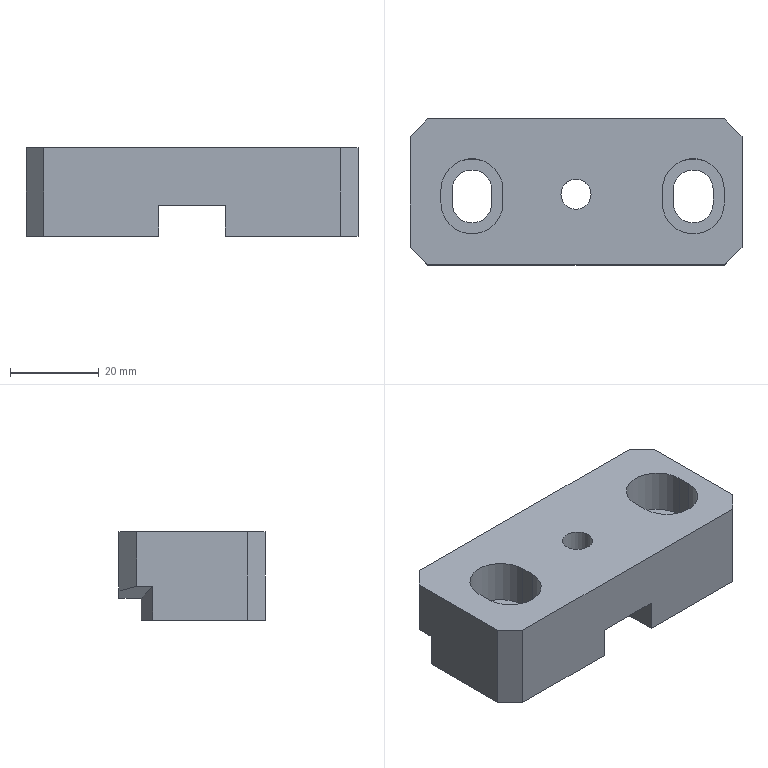Part | NX | features 20 2 | 1 solid | 41 faces | box 75 x 33 x 20 mm | volume 37493 mm3 | plane 32 | cylinder 9 | commonest cylinder face diameters 9 x4 14 x4 6.8 x1
STEP:
#1=CARTESIAN_POINT('',(1901.502,-433.5,16.5));
#2=VERTEX_POINT('',#1);
#3=CARTESIAN_POINT('',(1887.502,-433.5,16.5));
#4=VERTEX_POINT('',#3);
#5=CARTESIAN_POINT('',(1894.502,-433.5,16.5));
#6=DIRECTION('',(0.,0.,1.));
#7=DIRECTION('',(1.,0.,0.));
#8=AXIS2_PLACEMENT_3D('',#5,#6,#7);
#9=CIRCLE('',#8,7.);
#10=EDGE_CURVE('',#2,#4,#9,.T.);
#11=ORIENTED_EDGE('',*,*,#10,.F.);
#12=CARTESIAN_POINT('',(1901.502,-436.5,16.5));
#13=VERTEX_POINT('',#12);
#14=CARTESIAN_POINT('',(1901.502,-450.5,16.5));
#15=DIRECTION('',(0.,1.,0.));
#16=VECTOR('',#15,1000.);
#17=LINE('',#14,#16);
#18=EDGE_CURVE('',#13,#2,#17,.T.);
#19=ORIENTED_EDGE('',*,*,#18,.F.);
#20=CARTESIAN_POINT('',(1887.502,-436.5,16.5));
#21=VERTEX_POINT('',#20);
#22=CARTESIAN_POINT('',(1894.502,-436.5,16.5));
#23=DIRECTION('',(0.,0.,1.));
#24=DIRECTION('',(1.,0.,0.));
#25=AXIS2_PLACEMENT_3D('',#22,#23,#24);
#26=CIRCLE('',#25,7.);
#27=EDGE_CURVE('',#21,#13,#26,.T.);
#28=ORIENTED_EDGE('',*,*,#27,.F.);
#29=CARTESIAN_POINT('',(1887.502,-450.5,16.5));
#30=DIRECTION('',(0.,-1.,0.));
#31=VECTOR('',#30,1000.);
#32=LINE('',#29,#31);
#33=EDGE_CURVE('',#4,#21,#32,.T.);
#34=ORIENTED_EDGE('',*,*,#33,.F.);
#35=EDGE_LOOP('',(#11,#19,#28,#34));
#36=FACE_BOUND('',#35,.T.);
#37=CARTESIAN_POINT('',(1851.502,-436.5,16.5));
#38=VERTEX_POINT('',#37);
#39=CARTESIAN_POINT('',(1851.502,-433.5,16.5));
#40=VERTEX_POINT('',#39);
#41=CARTESIAN_POINT('',(1851.502,-450.5,16.5));
#42=DIRECTION('',(0.,1.,0.));
#43=VECTOR('',#42,1000.);
#44=LINE('',#41,#43);
#45=EDGE_CURVE('',#38,#40,#44,.T.);
#46=ORIENTED_EDGE('',*,*,#45,.F.);
#47=CARTESIAN_POINT('',(1837.502,-436.5,16.5));
#48=VERTEX_POINT('',#47);
#49=CARTESIAN_POINT('',(1844.502,-436.5,16.5));
#50=DIRECTION('',(0.,0.,1.));
#51=DIRECTION('',(1.,0.,0.));
#52=AXIS2_PLACEMENT_3D('',#49,#50,#51);
#53=CIRCLE('',#52,7.);
#54=EDGE_CURVE('',#48,#38,#53,.T.);
#55=ORIENTED_EDGE('',*,*,#54,.F.);
#56=CARTESIAN_POINT('',(1837.502,-433.5,16.5));
#57=VERTEX_POINT('',#56);
#58=CARTESIAN_POINT('',(1837.502,-450.5,16.5));
#59=DIRECTION('',(0.,-1.,0.));
#60=VECTOR('',#59,1000.);
#61=LINE('',#58,#60);
#62=EDGE_CURVE('',#57,#48,#61,.T.);
#63=ORIENTED_EDGE('',*,*,#62,.F.);
#64=CARTESIAN_POINT('',(1844.502,-433.5,16.5));
#65=DIRECTION('',(0.,0.,1.));
#66=DIRECTION('',(1.,0.,0.));
#67=AXIS2_PLACEMENT_3D('',#64,#65,#66);
#68=CIRCLE('',#67,7.);
#69=EDGE_CURVE('',#40,#57,#68,.T.);
#70=ORIENTED_EDGE('',*,*,#69,.F.);
#71=EDGE_LOOP('',(#46,#55,#63,#70));
#72=FACE_BOUND('',#71,.T.);
#73=CARTESIAN_POINT('',(1901.502,-417.5,16.5));
#74=VERTEX_POINT('',#73);
#75=CARTESIAN_POINT('',(1834.502,-417.5,16.5));
#76=VERTEX_POINT('',#75);
#77=CARTESIAN_POINT('',(1968.502,-417.5,16.5));
#78=DIRECTION('',(-1.,0.,0.));
#79=VECTOR('',#78,1000.);
#80=LINE('',#77,#79);
#81=EDGE_CURVE('',#74,#76,#80,.T.);
#82=ORIENTED_EDGE('',*,*,#81,.T.);
#83=CARTESIAN_POINT('',(1830.502,-421.5,16.5));
#84=VERTEX_POINT('',#83);
#85=CARTESIAN_POINT('',(1830.502,-421.5,16.5));
#86=DIRECTION('',(-0.7071,-0.7071,0.));
#87=VECTOR('',#86,1000.);
#88=LINE('',#85,#87);
#89=EDGE_CURVE('',#76,#84,#88,.T.);
#90=ORIENTED_EDGE('',*,*,#89,.T.);
#91=CARTESIAN_POINT('',(1830.502,-446.5,16.5));
#92=VERTEX_POINT('',#91);
#93=CARTESIAN_POINT('',(1830.502,-417.5,16.5));
#94=DIRECTION('',(0.,-1.,0.));
#95=VECTOR('',#94,1000.);
#96=LINE('',#93,#95);
#97=EDGE_CURVE('',#84,#92,#96,.T.);
#98=ORIENTED_EDGE('',*,*,#97,.T.);
#99=CARTESIAN_POINT('',(1834.502,-450.5,16.5));
#100=VERTEX_POINT('',#99);
#101=CARTESIAN_POINT('',(1834.502,-450.5,16.5));
#102=DIRECTION('',(0.7071,-0.7071,0.));
#103=VECTOR('',#102,1000.);
#104=LINE('',#101,#103);
#105=EDGE_CURVE('',#92,#100,#104,.T.);
#106=ORIENTED_EDGE('',*,*,#105,.T.);
#107=CARTESIAN_POINT('',(1901.502,-450.5,16.5));
#108=VERTEX_POINT('',#107);
#109=CARTESIAN_POINT('',(1888.502,-450.5,16.5));
#110=DIRECTION('',(1.,0.,0.));
#111=VECTOR('',#110,1000.);
#112=LINE('',#109,#111);
#113=EDGE_CURVE('',#100,#108,#112,.T.);
#114=ORIENTED_EDGE('',*,*,#113,.T.);
#115=CARTESIAN_POINT('',(1905.502,-446.5,16.5));
#116=VERTEX_POINT('',#115);
#117=CARTESIAN_POINT('',(1905.502,-446.5,16.5));
#118=DIRECTION('',(0.7071,0.7071,0.));
#119=VECTOR('',#118,1000.);
#120=LINE('',#117,#119);
#121=EDGE_CURVE('',#108,#116,#120,.T.);
#122=ORIENTED_EDGE('',*,*,#121,.T.);
#123=CARTESIAN_POINT('',(1905.502,-421.5,16.5));
#124=VERTEX_POINT('',#123);
#125=CARTESIAN_POINT('',(1905.502,-450.5,16.5));
#126=DIRECTION('',(0.,1.,0.));
#127=VECTOR('',#126,1000.);
#128=LINE('',#125,#127);
#129=EDGE_CURVE('',#116,#124,#128,.T.);
#130=ORIENTED_EDGE('',*,*,#129,.T.);
#131=CARTESIAN_POINT('',(1901.502,-417.5,16.5));
#132=DIRECTION('',(-0.7071,0.7071,0.));
#133=VECTOR('',#132,1000.);
#134=LINE('',#131,#133);
#135=EDGE_CURVE('',#124,#74,#134,.T.);
#136=ORIENTED_EDGE('',*,*,#135,.T.);
#137=EDGE_LOOP('',(#82,#90,#98,#106,#114,#122,#130,#136));
#138=FACE_BOUND('',#137,.T.);
#139=CARTESIAN_POINT('',(1871.402,-434.5,16.5));
#140=VERTEX_POINT('',#139);
#141=CARTESIAN_POINT('',(1868.002,-434.5,16.5));
#142=DIRECTION('',(0.,0.,-1.));
#143=DIRECTION('',(1.,0.,0.));
#144=AXIS2_PLACEMENT_3D('',#141,#142,#143);
#145=CIRCLE('',#144,3.4);
#146=EDGE_CURVE('',#140,#140,#145,.T.);
#147=ORIENTED_EDGE('',*,*,#146,.T.);
#148=EDGE_LOOP('',(#147));
#149=FACE_BOUND('',#148,.T.);
#150=CARTESIAN_POINT('',(1968.502,-450.5,16.5));
#151=DIRECTION('',(0.,0.,1.));
#152=DIRECTION('',(-1.,0.,0.));
#153=AXIS2_PLACEMENT_3D('',#150,#151,#152);
#154=PLANE('',#153);
#155=ADVANCED_FACE('',(#36,#72,#138,#149),#154,.T.);
#156=CARTESIAN_POINT('',(1875.502,-417.5,3.5));
#157=VERTEX_POINT('',#156);
#158=CARTESIAN_POINT('',(1875.502,-450.5,3.5));
#159=VERTEX_POINT('',#158);
#160=CARTESIAN_POINT('',(1875.502,-436.5,3.5));
#161=DIRECTION('',(0.,-1.,0.));
#162=VECTOR('',#161,1000.);
#163=LINE('',#160,#162);
#164=EDGE_CURVE('',#157,#159,#163,.T.);
#165=ORIENTED_EDGE('',*,*,#164,.F.);
#166=CARTESIAN_POINT('',(1875.502,-417.5,1.5));
#167=VERTEX_POINT('',#166);
#168=CARTESIAN_POINT('',(1875.502,-417.5,11.5));
#169=DIRECTION('',(0.,0.,-1.));
#170=VECTOR('',#169,1000.);
#171=LINE('',#168,#170);
#172=EDGE_CURVE('',#157,#167,#171,.T.);
#173=ORIENTED_EDGE('',*,*,#172,.T.);
#174=CARTESIAN_POINT('',(1875.502,-422.5,1.5));
#175=VERTEX_POINT('',#174);
#176=CARTESIAN_POINT('',(1875.502,-396.891,1.5));
#177=DIRECTION('',(0.,1.,0.));
#178=VECTOR('',#177,1000.);
#179=LINE('',#176,#178);
#180=EDGE_CURVE('',#175,#167,#179,.T.);
#181=ORIENTED_EDGE('',*,*,#180,.F.);
#182=CARTESIAN_POINT('',(1875.502,-422.5,-3.5));
#183=VERTEX_POINT('',#182);
#184=CARTESIAN_POINT('',(1875.502,-422.5,3.5));
#185=DIRECTION('',(0.,0.,-1.));
#186=VECTOR('',#185,1000.);
#187=LINE('',#184,#186);
#188=EDGE_CURVE('',#175,#183,#187,.T.);
#189=ORIENTED_EDGE('',*,*,#188,.T.);
#190=CARTESIAN_POINT('',(1875.502,-450.5,-3.5));
#191=VERTEX_POINT('',#190);
#192=CARTESIAN_POINT('',(1875.502,-450.5,-3.5));
#193=DIRECTION('',(0.,-1.,0.));
#194=VECTOR('',#193,1000.);
#195=LINE('',#192,#194);
#196=EDGE_CURVE('',#183,#191,#195,.T.);
#197=ORIENTED_EDGE('',*,*,#196,.T.);
#198=CARTESIAN_POINT('',(1875.502,-450.5,11.5));
#199=DIRECTION('',(0.,0.,1.));
#200=VECTOR('',#199,1000.);
#201=LINE('',#198,#200);
#202=EDGE_CURVE('',#191,#159,#201,.T.);
#203=ORIENTED_EDGE('',*,*,#202,.T.);
#204=EDGE_LOOP('',(#165,#173,#181,#189,#197,#203));
#205=FACE_BOUND('',#204,.T.);
#206=CARTESIAN_POINT('',(1875.502,-436.5,0.));
#207=DIRECTION('',(-1.,0.,0.));
#208=DIRECTION('',(0.,0.,1.));
#209=AXIS2_PLACEMENT_3D('',#206,#207,#208);
#210=PLANE('',#209);
#211=ADVANCED_FACE('',(#205),#210,.T.);
#212=CARTESIAN_POINT('',(1860.502,-422.5,-3.5));
#213=VERTEX_POINT('',#212);
#214=CARTESIAN_POINT('',(1860.502,-450.5,-3.5));
#215=VERTEX_POINT('',#214);
#216=CARTESIAN_POINT('',(1860.502,-450.5,-3.5));
#217=DIRECTION('',(0.,-1.,0.));
#218=VECTOR('',#217,1000.);
#219=LINE('',#216,#218);
#220=EDGE_CURVE('',#213,#215,#219,.T.);
#221=ORIENTED_EDGE('',*,*,#220,.F.);
#222=CARTESIAN_POINT('',(1860.502,-422.5,1.5));
#223=VERTEX_POINT('',#222);
#224=CARTESIAN_POINT('',(1860.502,-422.5,3.5));
#225=DIRECTION('',(0.,0.,-1.));
#226=VECTOR('',#225,1000.);
#227=LINE('',#224,#226);
#228=EDGE_CURVE('',#223,#213,#227,.T.);
#229=ORIENTED_EDGE('',*,*,#228,.F.);
#230=CARTESIAN_POINT('',(1860.502,-417.5,1.5));
#231=VERTEX_POINT('',#230);
#232=CARTESIAN_POINT('',(1860.502,-396.891,1.5));
#233=DIRECTION('',(0.,1.,0.));
#234=VECTOR('',#233,1000.);
#235=LINE('',#232,#234);
#236=EDGE_CURVE('',#223,#231,#235,.T.);
#237=ORIENTED_EDGE('',*,*,#236,.T.);
#238=CARTESIAN_POINT('',(1860.502,-417.5,3.5));
#239=VERTEX_POINT('',#238);
#240=CARTESIAN_POINT('',(1860.502,-417.5,11.5));
#241=DIRECTION('',(0.,0.,-1.));
#242=VECTOR('',#241,1000.);
#243=LINE('',#240,#242);
#244=EDGE_CURVE('',#239,#231,#243,.T.);
#245=ORIENTED_EDGE('',*,*,#244,.F.);
#246=CARTESIAN_POINT('',(1860.502,-450.5,3.5));
#247=VERTEX_POINT('',#246);
#248=CARTESIAN_POINT('',(1860.502,-436.5,3.5));
#249=DIRECTION('',(0.,1.,0.));
#250=VECTOR('',#249,1000.);
#251=LINE('',#248,#250);
#252=EDGE_CURVE('',#247,#239,#251,.T.);
#253=ORIENTED_EDGE('',*,*,#252,.F.);
#254=CARTESIAN_POINT('',(1860.502,-450.5,11.5));
#255=DIRECTION('',(0.,0.,1.));
#256=VECTOR('',#255,1000.);
#257=LINE('',#254,#256);
#258=EDGE_CURVE('',#215,#247,#257,.T.);
#259=ORIENTED_EDGE('',*,*,#258,.F.);
#260=EDGE_LOOP('',(#221,#229,#237,#245,#253,#259));
#261=FACE_BOUND('',#260,.T.);
#262=CARTESIAN_POINT('',(1860.502,-436.5,-9.5));
#263=DIRECTION('',(-1.,0.,0.));
#264=DIRECTION('',(0.,0.,-1.));
#265=AXIS2_PLACEMENT_3D('',#262,#263,#264);
#266=PLANE('',#265);
#267=ADVANCED_FACE('',(#261),#266,.F.);
#268=CARTESIAN_POINT('',(1871.402,-434.5,3.5));
#269=VERTEX_POINT('',#268);
#270=CARTESIAN_POINT('',(1868.002,-434.5,3.5));
#271=DIRECTION('',(0.,0.,1.));
#272=DIRECTION('',(1.,0.,0.));
#273=AXIS2_PLACEMENT_3D('',#270,#271,#272);
#274=CIRCLE('',#273,3.4);
#275=EDGE_CURVE('',#269,#269,#274,.T.);
#276=ORIENTED_EDGE('',*,*,#275,.T.);
#277=EDGE_LOOP('',(#276));
#278=FACE_BOUND('',#277,.T.);
#279=CARTESIAN_POINT('',(1938.502,-450.5,3.5));
#280=DIRECTION('',(1.,0.,0.));
#281=VECTOR('',#280,1000.);
#282=LINE('',#279,#281);
#283=EDGE_CURVE('',#247,#159,#282,.T.);
#284=ORIENTED_EDGE('',*,*,#283,.F.);
#285=ORIENTED_EDGE('',*,*,#252,.T.);
#286=CARTESIAN_POINT('',(2018.502,-417.5,3.5));
#287=DIRECTION('',(-1.,0.,0.));
#288=VECTOR('',#287,1000.);
#289=LINE('',#286,#288);
#290=EDGE_CURVE('',#157,#239,#289,.T.);
#291=ORIENTED_EDGE('',*,*,#290,.F.);
#292=ORIENTED_EDGE('',*,*,#164,.T.);
#293=EDGE_LOOP('',(#284,#285,#291,#292));
#294=FACE_BOUND('',#293,.T.);
#295=CARTESIAN_POINT('',(1868.002,-436.5,3.5));
#296=DIRECTION('',(0.,0.,1.));
#297=DIRECTION('',(0.,-1.,0.));
#298=AXIS2_PLACEMENT_3D('',#295,#296,#297);
#299=PLANE('',#298);
#300=ADVANCED_FACE('',(#278,#294),#299,.F.);
#301=CARTESIAN_POINT('',(1890.002,-436.5,6.5));
#302=VERTEX_POINT('',#301);
#303=CARTESIAN_POINT('',(1890.002,-433.5,6.5));
#304=VERTEX_POINT('',#303);
#305=CARTESIAN_POINT('',(1890.002,-432.5,6.5));
#306=DIRECTION('',(0.,1.,0.));
#307=VECTOR('',#306,1000.);
#308=LINE('',#305,#307);
#309=EDGE_CURVE('',#302,#304,#308,.T.);
#310=ORIENTED_EDGE('',*,*,#309,.T.);
#311=CARTESIAN_POINT('',(1899.002,-433.5,6.5));
#312=VERTEX_POINT('',#311);
#313=CARTESIAN_POINT('',(1894.502,-433.5,6.5));
#314=DIRECTION('',(0.,0.,-1.));
#315=DIRECTION('',(-1.,0.,0.));
#316=AXIS2_PLACEMENT_3D('',#313,#314,#315);
#317=CIRCLE('',#316,4.5);
#318=EDGE_CURVE('',#304,#312,#317,.T.);
#319=ORIENTED_EDGE('',*,*,#318,.T.);
#320=CARTESIAN_POINT('',(1899.002,-436.5,6.5));
#321=VERTEX_POINT('',#320);
#322=CARTESIAN_POINT('',(1899.002,-439.5,6.5));
#323=DIRECTION('',(0.,-1.,0.));
#324=VECTOR('',#323,1000.);
#325=LINE('',#322,#324);
#326=EDGE_CURVE('',#312,#321,#325,.T.);
#327=ORIENTED_EDGE('',*,*,#326,.T.);
#328=CARTESIAN_POINT('',(1894.502,-436.5,6.5));
#329=DIRECTION('',(0.,0.,-1.));
#330=DIRECTION('',(-1.,0.,0.));
#331=AXIS2_PLACEMENT_3D('',#328,#329,#330);
#332=CIRCLE('',#331,4.5);
#333=EDGE_CURVE('',#321,#302,#332,.T.);
#334=ORIENTED_EDGE('',*,*,#333,.T.);
#335=EDGE_LOOP('',(#310,#319,#327,#334));
#336=FACE_BOUND('',#335,.T.);
#337=CARTESIAN_POINT('',(1901.502,-433.5,6.5));
#338=VERTEX_POINT('',#337);
#339=CARTESIAN_POINT('',(1887.502,-433.5,6.5));
#340=VERTEX_POINT('',#339);
#341=CARTESIAN_POINT('',(1894.502,-433.5,6.5));
#342=DIRECTION('',(0.,0.,1.));
#343=DIRECTION('',(-1.,0.,0.));
#344=AXIS2_PLACEMENT_3D('',#341,#342,#343);
#345=CIRCLE('',#344,7.);
#346=EDGE_CURVE('',#338,#340,#345,.T.);
#347=ORIENTED_EDGE('',*,*,#346,.T.);
#348=CARTESIAN_POINT('',(1887.502,-436.5,6.5));
#349=VERTEX_POINT('',#348);
#350=CARTESIAN_POINT('',(1887.502,-439.5,6.5));
#351=DIRECTION('',(0.,-1.,0.));
#352=VECTOR('',#351,1000.);
#353=LINE('',#350,#352);
#354=EDGE_CURVE('',#340,#349,#353,.T.);
#355=ORIENTED_EDGE('',*,*,#354,.T.);
#356=CARTESIAN_POINT('',(1901.502,-436.5,6.5));
#357=VERTEX_POINT('',#356);
#358=CARTESIAN_POINT('',(1894.502,-436.5,6.5));
#359=DIRECTION('',(0.,0.,1.));
#360=DIRECTION('',(-1.,0.,0.));
#361=AXIS2_PLACEMENT_3D('',#358,#359,#360);
#362=CIRCLE('',#361,7.);
#363=EDGE_CURVE('',#349,#357,#362,.T.);
#364=ORIENTED_EDGE('',*,*,#363,.T.);
#365=CARTESIAN_POINT('',(1901.502,-432.5,6.5));
#366=DIRECTION('',(0.,1.,0.));
#367=VECTOR('',#366,1000.);
#368=LINE('',#365,#367);
#369=EDGE_CURVE('',#357,#338,#368,.T.);
#370=ORIENTED_EDGE('',*,*,#369,.T.);
#371=EDGE_LOOP('',(#347,#355,#364,#370));
#372=FACE_BOUND('',#371,.T.);
#373=CARTESIAN_POINT('',(1894.502,-432.5,6.5));
#374=DIRECTION('',(0.,0.,-1.));
#375=DIRECTION('',(1.,0.,0.));
#376=AXIS2_PLACEMENT_3D('',#373,#374,#375);
#377=PLANE('',#376);
#378=ADVANCED_FACE('',(#336,#372),#377,.F.);
#379=CARTESIAN_POINT('',(1895.502,-417.5,1.5));
#380=VERTEX_POINT('',#379);
#381=CARTESIAN_POINT('',(1895.502,-422.5,1.5));
#382=VERTEX_POINT('',#381);
#383=CARTESIAN_POINT('',(1895.502,-425.18,1.5));
#384=DIRECTION('',(0.,-1.,0.));
#385=VECTOR('',#384,1000.);
#386=LINE('',#383,#385);
#387=EDGE_CURVE('',#380,#382,#386,.T.);
#388=ORIENTED_EDGE('',*,*,#387,.F.);
#389=CARTESIAN_POINT('',(1901.502,-417.5,3.108));
#390=VERTEX_POINT('',#389);
#391=CARTESIAN_POINT('',(1895.502,-417.5,1.5));
#392=DIRECTION('',(-0.9659,0.,-0.2588));
#393=VECTOR('',#392,1000.);
#394=LINE('',#391,#393);
#395=EDGE_CURVE('',#390,#380,#394,.T.);
#396=ORIENTED_EDGE('',*,*,#395,.F.);
#397=CARTESIAN_POINT('',(1905.502,-421.5,4.179));
#398=VERTEX_POINT('',#397);
#399=CARTESIAN_POINT('',(1888.451,-404.449,-0.3894));
#400=DIRECTION('',(0.6947,-0.6947,0.1862));
#401=VECTOR('',#400,1000.);
#402=LINE('',#399,#401);
#403=EDGE_CURVE('',#390,#398,#402,.T.);
#404=ORIENTED_EDGE('',*,*,#403,.T.);
#405=CARTESIAN_POINT('',(1905.502,-425.18,4.179));
#406=VERTEX_POINT('',#405);
#407=CARTESIAN_POINT('',(1905.502,-417.5,4.179));
#408=DIRECTION('',(0.,1.,0.));
#409=VECTOR('',#408,1000.);
#410=LINE('',#407,#409);
#411=EDGE_CURVE('',#406,#398,#410,.T.);
#412=ORIENTED_EDGE('',*,*,#411,.F.);
#413=CARTESIAN_POINT('',(1904.875,-425.012,4.011));
#414=DIRECTION('',(0.9351,-0.2506,0.2506));
#415=VECTOR('',#414,1000.);
#416=LINE('',#413,#415);
#417=EDGE_CURVE('',#382,#406,#416,.T.);
#418=ORIENTED_EDGE('',*,*,#417,.F.);
#419=EDGE_LOOP('',(#388,#396,#404,#412,#418));
#420=FACE_BOUND('',#419,.T.);
#421=CARTESIAN_POINT('',(1895.502,-396.891,1.5));
#422=DIRECTION('',(0.2588,0.,-0.9659));
#423=DIRECTION('',(0.9659,0.,0.2588));
#424=AXIS2_PLACEMENT_3D('',#421,#422,#423);
#425=PLANE('',#424);
#426=ADVANCED_FACE('',(#420),#425,.T.);
#427=CARTESIAN_POINT('',(1849.002,-433.5,6.5));
#428=VERTEX_POINT('',#427);
#429=CARTESIAN_POINT('',(1849.002,-436.5,6.5));
#430=VERTEX_POINT('',#429);
#431=CARTESIAN_POINT('',(1849.002,-432.5,6.5));
#432=DIRECTION('',(0.,-1.,0.));
#433=VECTOR('',#432,1000.);
#434=LINE('',#431,#433);
#435=EDGE_CURVE('',#428,#430,#434,.T.);
#436=ORIENTED_EDGE('',*,*,#435,.T.);
#437=CARTESIAN_POINT('',(1840.002,-436.5,6.5));
#438=VERTEX_POINT('',#437);
#439=CARTESIAN_POINT('',(1844.502,-436.5,6.5));
#440=DIRECTION('',(0.,0.,-1.));
#441=DIRECTION('',(-1.,0.,0.));
#442=AXIS2_PLACEMENT_3D('',#439,#440,#441);
#443=CIRCLE('',#442,4.5);
#444=EDGE_CURVE('',#430,#438,#443,.T.);
#445=ORIENTED_EDGE('',*,*,#444,.T.);
#446=CARTESIAN_POINT('',(1840.002,-433.5,6.5));
#447=VERTEX_POINT('',#446);
#448=CARTESIAN_POINT('',(1840.002,-439.5,6.5));
#449=DIRECTION('',(0.,1.,0.));
#450=VECTOR('',#449,1000.);
#451=LINE('',#448,#450);
#452=EDGE_CURVE('',#438,#447,#451,.T.);
#453=ORIENTED_EDGE('',*,*,#452,.T.);
#454=CARTESIAN_POINT('',(1844.502,-433.5,6.5));
#455=DIRECTION('',(0.,0.,-1.));
#456=DIRECTION('',(-1.,0.,0.));
#457=AXIS2_PLACEMENT_3D('',#454,#455,#456);
#458=CIRCLE('',#457,4.5);
#459=EDGE_CURVE('',#447,#428,#458,.T.);
#460=ORIENTED_EDGE('',*,*,#459,.T.);
#461=EDGE_LOOP('',(#436,#445,#453,#460));
#462=FACE_BOUND('',#461,.T.);
#463=CARTESIAN_POINT('',(1851.502,-433.5,6.5));
#464=VERTEX_POINT('',#463);
#465=CARTESIAN_POINT('',(1837.502,-433.5,6.5));
#466=VERTEX_POINT('',#465);
#467=CARTESIAN_POINT('',(1844.502,-433.5,6.5));
#468=DIRECTION('',(0.,0.,1.));
#469=DIRECTION('',(-1.,0.,0.));
#470=AXIS2_PLACEMENT_3D('',#467,#468,#469);
#471=CIRCLE('',#470,7.);
#472=EDGE_CURVE('',#464,#466,#471,.T.);
#473=ORIENTED_EDGE('',*,*,#472,.T.);
#474=CARTESIAN_POINT('',(1837.502,-436.5,6.5));
#475=VERTEX_POINT('',#474);
#476=CARTESIAN_POINT('',(1837.502,-432.5,6.5));
#477=DIRECTION('',(0.,-1.,0.));
#478=VECTOR('',#477,1000.);
#479=LINE('',#476,#478);
#480=EDGE_CURVE('',#466,#475,#479,.T.);
#481=ORIENTED_EDGE('',*,*,#480,.T.);
#482=CARTESIAN_POINT('',(1851.502,-436.5,6.5));
#483=VERTEX_POINT('',#482);
#484=CARTESIAN_POINT('',(1844.502,-436.5,6.5));
#485=DIRECTION('',(0.,0.,1.));
#486=DIRECTION('',(-1.,0.,0.));
#487=AXIS2_PLACEMENT_3D('',#484,#485,#486);
#488=CIRCLE('',#487,7.);
#489=EDGE_CURVE('',#475,#483,#488,.T.);
#490=ORIENTED_EDGE('',*,*,#489,.T.);
#491=CARTESIAN_POINT('',(1851.502,-439.5,6.5));
#492=DIRECTION('',(0.,1.,0.));
#493=VECTOR('',#492,1000.);
#494=LINE('',#491,#493);
#495=EDGE_CURVE('',#483,#464,#494,.T.);
#496=ORIENTED_EDGE('',*,*,#495,.T.);
#497=EDGE_LOOP('',(#473,#481,#490,#496));
#498=FACE_BOUND('',#497,.T.);
#499=CARTESIAN_POINT('',(1844.502,-432.5,6.5));
#500=DIRECTION('',(0.,0.,-1.));
#501=DIRECTION('',(-1.,0.,0.));
#502=AXIS2_PLACEMENT_3D('',#499,#500,#501);
#503=PLANE('',#502);
#504=ADVANCED_FACE('',(#462,#498),#503,.F.);
#505=ORIENTED_EDGE('',*,*,#33,.T.);
#506=CARTESIAN_POINT('',(1887.502,-436.5,42.5));
#507=DIRECTION('',(0.,0.,1.));
#508=VECTOR('',#507,1000.);
#509=LINE('',#506,#508);
#510=EDGE_CURVE('',#349,#21,#509,.T.);
#511=ORIENTED_EDGE('',*,*,#510,.F.);
#512=ORIENTED_EDGE('',*,*,#354,.F.);
#513=CARTESIAN_POINT('',(1887.502,-433.5,42.5));
#514=DIRECTION('',(0.,0.,1.));
#515=VECTOR('',#514,1000.);
#516=LINE('',#513,#515);
#517=EDGE_CURVE('',#340,#4,#516,.T.);
#518=ORIENTED_EDGE('',*,*,#517,.T.);
#519=EDGE_LOOP('',(#505,#511,#512,#518));
#520=FACE_BOUND('',#519,.T.);
#521=CARTESIAN_POINT('',(1887.502,-439.5,42.5));
#522=DIRECTION('',(-1.,0.,0.));
#523=DIRECTION('',(0.,0.,-1.));
#524=AXIS2_PLACEMENT_3D('',#521,#522,#523);
#525=PLANE('',#524);
#526=ADVANCED_FACE('',(#520),#525,.F.);
#527=ORIENTED_EDGE('',*,*,#27,.T.);
#528=CARTESIAN_POINT('',(1901.502,-436.5,42.5));
#529=DIRECTION('',(0.,0.,1.));
#530=VECTOR('',#529,1000.);
#531=LINE('',#528,#530);
#532=EDGE_CURVE('',#357,#13,#531,.T.);
#533=ORIENTED_EDGE('',*,*,#532,.F.);
#534=ORIENTED_EDGE('',*,*,#363,.F.);
#535=ORIENTED_EDGE('',*,*,#510,.T.);
#536=EDGE_LOOP('',(#527,#533,#534,#535));
#537=FACE_BOUND('',#536,.T.);
#538=CARTESIAN_POINT('',(1894.502,-436.5,42.5));
#539=DIRECTION('',(0.,0.,-1.));
#540=DIRECTION('',(1.,0.,0.));
#541=AXIS2_PLACEMENT_3D('',#538,#539,#540);
#542=CYLINDRICAL_SURFACE('',#541,7.);
#543=ADVANCED_FACE('',(#537),#542,.F.);
#544=ORIENTED_EDGE('',*,*,#18,.T.);
#545=CARTESIAN_POINT('',(1901.502,-433.5,42.5));
#546=DIRECTION('',(0.,0.,1.));
#547=VECTOR('',#546,1000.);
#548=LINE('',#545,#547);
#549=EDGE_CURVE('',#338,#2,#548,.T.);
#550=ORIENTED_EDGE('',*,*,#549,.F.);
#551=ORIENTED_EDGE('',*,*,#369,.F.);
#552=ORIENTED_EDGE('',*,*,#532,.T.);
#553=EDGE_LOOP('',(#544,#550,#551,#552));
#554=FACE_BOUND('',#553,.T.);
#555=CARTESIAN_POINT('',(1901.502,-432.5,42.5));
#556=DIRECTION('',(1.,0.,0.));
#557=DIRECTION('',(0.,0.,1.));
#558=AXIS2_PLACEMENT_3D('',#555,#556,#557);
#559=PLANE('',#558);
#560=ADVANCED_FACE('',(#554),#559,.F.);
#561=ORIENTED_EDGE('',*,*,#10,.T.);
#562=ORIENTED_EDGE('',*,*,#517,.F.);
#563=ORIENTED_EDGE('',*,*,#346,.F.);
#564=ORIENTED_EDGE('',*,*,#549,.T.);
#565=EDGE_LOOP('',(#561,#562,#563,#564));
#566=FACE_BOUND('',#565,.T.);
#567=CARTESIAN_POINT('',(1894.502,-433.5,42.5));
#568=DIRECTION('',(0.,0.,-1.));
#569=DIRECTION('',(1.,0.,0.));
#570=AXIS2_PLACEMENT_3D('',#567,#568,#569);
#571=CYLINDRICAL_SURFACE('',#570,7.);
#572=ADVANCED_FACE('',(#566),#571,.F.);
#573=ORIENTED_EDGE('',*,*,#135,.F.);
#574=CARTESIAN_POINT('',(1905.502,-421.5,11.5));
#575=DIRECTION('',(0.,0.,1.));
#576=VECTOR('',#575,1000.);
#577=LINE('',#574,#576);
#578=EDGE_CURVE('',#398,#124,#577,.T.);
#579=ORIENTED_EDGE('',*,*,#578,.F.);
#580=ORIENTED_EDGE('',*,*,#403,.F.);
#581=CARTESIAN_POINT('',(1901.502,-417.5,11.5));
#582=DIRECTION('',(0.,0.,-1.));
#583=VECTOR('',#582,1000.);
#584=LINE('',#581,#583);
#585=EDGE_CURVE('',#74,#390,#584,.T.);
#586=ORIENTED_EDGE('',*,*,#585,.F.);
#587=EDGE_LOOP('',(#573,#579,#580,#586));
#588=FACE_BOUND('',#587,.T.);
#589=CARTESIAN_POINT('',(1901.502,-417.5,11.5));
#590=DIRECTION('',(-0.7071,-0.7071,0.));
#591=DIRECTION('',(0.,0.,-1.));
#592=AXIS2_PLACEMENT_3D('',#589,#590,#591);
#593=PLANE('',#592);
#594=ADVANCED_FACE('',(#588),#593,.F.);
#595=ORIENTED_EDGE('',*,*,#69,.T.);
#596=CARTESIAN_POINT('',(1837.502,-433.5,42.5));
#597=DIRECTION('',(0.,0.,-1.));
#598=VECTOR('',#597,1000.);
#599=LINE('',#596,#598);
#600=EDGE_CURVE('',#57,#466,#599,.T.);
#601=ORIENTED_EDGE('',*,*,#600,.T.);
#602=ORIENTED_EDGE('',*,*,#472,.F.);
#603=CARTESIAN_POINT('',(1851.502,-433.5,42.5));
#604=DIRECTION('',(0.,0.,-1.));
#605=VECTOR('',#604,1000.);
#606=LINE('',#603,#605);
#607=EDGE_CURVE('',#40,#464,#606,.T.);
#608=ORIENTED_EDGE('',*,*,#607,.F.);
#609=EDGE_LOOP('',(#595,#601,#602,#608));
#610=FACE_BOUND('',#609,.T.);
#611=CARTESIAN_POINT('',(1844.502,-433.5,42.5));
#612=DIRECTION('',(0.,0.,-1.));
#613=DIRECTION('',(-1.,0.,0.));
#614=AXIS2_PLACEMENT_3D('',#611,#612,#613);
#615=CYLINDRICAL_SURFACE('',#614,7.);
#616=ADVANCED_FACE('',(#610),#615,.F.);
#617=ORIENTED_EDGE('',*,*,#62,.T.);
#618=CARTESIAN_POINT('',(1837.502,-436.5,42.5));
#619=DIRECTION('',(0.,0.,-1.));
#620=VECTOR('',#619,1000.);
#621=LINE('',#618,#620);
#622=EDGE_CURVE('',#48,#475,#621,.T.);
#623=ORIENTED_EDGE('',*,*,#622,.T.);
#624=ORIENTED_EDGE('',*,*,#480,.F.);
#625=ORIENTED_EDGE('',*,*,#600,.F.);
#626=EDGE_LOOP('',(#617,#623,#624,#625));
#627=FACE_BOUND('',#626,.T.);
#628=CARTESIAN_POINT('',(1837.502,-432.5,42.5));
#629=DIRECTION('',(-1.,0.,0.));
#630=DIRECTION('',(0.,0.,1.));
#631=AXIS2_PLACEMENT_3D('',#628,#629,#630);
#632=PLANE('',#631);
#633=ADVANCED_FACE('',(#627),#632,.F.);
#634=ORIENTED_EDGE('',*,*,#54,.T.);
#635=CARTESIAN_POINT('',(1851.502,-436.5,42.5));
#636=DIRECTION('',(0.,0.,-1.));
#637=VECTOR('',#636,1000.);
#638=LINE('',#635,#637);
#639=EDGE_CURVE('',#38,#483,#638,.T.);
#640=ORIENTED_EDGE('',*,*,#639,.T.);
#641=ORIENTED_EDGE('',*,*,#489,.F.);
#642=ORIENTED_EDGE('',*,*,#622,.F.);
#643=EDGE_LOOP('',(#634,#640,#641,#642));
#644=FACE_BOUND('',#643,.T.);
#645=CARTESIAN_POINT('',(1844.502,-436.5,42.5));
#646=DIRECTION('',(0.,0.,-1.));
#647=DIRECTION('',(-1.,0.,0.));
#648=AXIS2_PLACEMENT_3D('',#645,#646,#647);
#649=CYLINDRICAL_SURFACE('',#648,7.);
#650=ADVANCED_FACE('',(#644),#649,.F.);
#651=ORIENTED_EDGE('',*,*,#45,.T.);
#652=ORIENTED_EDGE('',*,*,#607,.T.);
#653=ORIENTED_EDGE('',*,*,#495,.F.);
#654=ORIENTED_EDGE('',*,*,#639,.F.);
#655=EDGE_LOOP('',(#651,#652,#653,#654));
#656=FACE_BOUND('',#655,.T.);
#657=CARTESIAN_POINT('',(1851.502,-439.5,42.5));
#658=DIRECTION('',(1.,0.,0.));
#659=DIRECTION('',(0.,0.,-1.));
#660=AXIS2_PLACEMENT_3D('',#657,#658,#659);
#661=PLANE('',#660);
#662=ADVANCED_FACE('',(#656),#661,.F.);
#663=ORIENTED_EDGE('',*,*,#411,.T.);
#664=ORIENTED_EDGE('',*,*,#578,.T.);
#665=ORIENTED_EDGE('',*,*,#129,.F.);
#666=CARTESIAN_POINT('',(1905.502,-446.5,-3.5));
#667=VERTEX_POINT('',#666);
#668=CARTESIAN_POINT('',(1905.502,-446.5,11.5));
#669=DIRECTION('',(0.,0.,-1.));
#670=VECTOR('',#669,1000.);
#671=LINE('',#668,#670);
#672=EDGE_CURVE('',#116,#667,#671,.T.);
#673=ORIENTED_EDGE('',*,*,#672,.T.);
#674=CARTESIAN_POINT('',(1905.502,-425.18,-3.5));
#675=VERTEX_POINT('',#674);
#676=CARTESIAN_POINT('',(1905.502,-450.5,-3.5));
#677=DIRECTION('',(0.,1.,0.));
#678=VECTOR('',#677,1000.);
#679=LINE('',#676,#678);
#680=EDGE_CURVE('',#667,#675,#679,.T.);
#681=ORIENTED_EDGE('',*,*,#680,.T.);
#682=CARTESIAN_POINT('',(1905.502,-425.18,3.5));
#683=DIRECTION('',(0.,0.,-1.));
#684=VECTOR('',#683,1000.);
#685=LINE('',#682,#684);
#686=EDGE_CURVE('',#406,#675,#685,.T.);
#687=ORIENTED_EDGE('',*,*,#686,.F.);
#688=EDGE_LOOP('',(#663,#664,#665,#673,#681,#687));
#689=FACE_BOUND('',#688,.T.);
#690=CARTESIAN_POINT('',(1905.502,-450.5,11.5));
#691=DIRECTION('',(-1.,0.,0.));
#692=DIRECTION('',(0.,0.,-1.));
#693=AXIS2_PLACEMENT_3D('',#690,#691,#692);
#694=PLANE('',#693);
#695=ADVANCED_FACE('',(#689),#694,.F.);
#696=CARTESIAN_POINT('',(1895.501,-422.5,1.5));
#697=VERTEX_POINT('',#696);
#698=CARTESIAN_POINT('',(1905.502,-425.18,1.5));
#699=DIRECTION('',(0.9659,-0.2588,0.));
#700=VECTOR('',#699,1000.);
#701=LINE('',#698,#700);
#702=EDGE_CURVE('',#697,#382,#701,.T.);
#703=ORIENTED_EDGE('',*,*,#702,.T.);
#704=ORIENTED_EDGE('',*,*,#417,.T.);
#705=ORIENTED_EDGE('',*,*,#686,.T.);
#706=CARTESIAN_POINT('',(1895.501,-422.5,-3.5));
#707=VERTEX_POINT('',#706);
#708=CARTESIAN_POINT('',(1905.502,-425.18,-3.5));
#709=DIRECTION('',(-0.9659,0.2588,0.));
#710=VECTOR('',#709,1000.);
#711=LINE('',#708,#710);
#712=EDGE_CURVE('',#675,#707,#711,.T.);
#713=ORIENTED_EDGE('',*,*,#712,.T.);
#714=CARTESIAN_POINT('',(1895.501,-422.5,3.5));
#715=DIRECTION('',(0.,0.,1.));
#716=VECTOR('',#715,1000.);
#717=LINE('',#714,#716);
#718=EDGE_CURVE('',#707,#697,#717,.T.);
#719=ORIENTED_EDGE('',*,*,#718,.T.);
#720=EDGE_LOOP('',(#703,#704,#705,#713,#719));
#721=FACE_BOUND('',#720,.T.);
#722=CARTESIAN_POINT('',(1905.502,-425.18,3.5));
#723=DIRECTION('',(-0.2588,-0.9659,0.));
#724=DIRECTION('',(0.9659,-0.2588,0.));
#725=AXIS2_PLACEMENT_3D('',#722,#723,#724);
#726=PLANE('',#725);
#727=ADVANCED_FACE('',(#721),#726,.F.);
#728=ORIENTED_EDGE('',*,*,#318,.F.);
#729=CARTESIAN_POINT('',(1890.002,-433.5,-3.5));
#730=VERTEX_POINT('',#729);
#731=CARTESIAN_POINT('',(1890.002,-433.5,42.5));
#732=DIRECTION('',(0.,0.,1.));
#733=VECTOR('',#732,1000.);
#734=LINE('',#731,#733);
#735=EDGE_CURVE('',#730,#304,#734,.T.);
#736=ORIENTED_EDGE('',*,*,#735,.F.);
#737=CARTESIAN_POINT('',(1899.002,-433.5,-3.5));
#738=VERTEX_POINT('',#737);
#739=CARTESIAN_POINT('',(1894.502,-433.5,-3.5));
#740=DIRECTION('',(0.,0.,1.));
#741=DIRECTION('',(1.,0.,0.));
#742=AXIS2_PLACEMENT_3D('',#739,#740,#741);
#743=CIRCLE('',#742,4.5);
#744=EDGE_CURVE('',#738,#730,#743,.T.);
#745=ORIENTED_EDGE('',*,*,#744,.F.);
#746=CARTESIAN_POINT('',(1899.002,-433.5,42.5));
#747=DIRECTION('',(0.,0.,1.));
#748=VECTOR('',#747,1000.);
#749=LINE('',#746,#748);
#750=EDGE_CURVE('',#738,#312,#749,.T.);
#751=ORIENTED_EDGE('',*,*,#750,.T.);
#752=EDGE_LOOP('',(#728,#736,#745,#751));
#753=FACE_BOUND('',#752,.T.);
#754=CARTESIAN_POINT('',(1894.502,-433.5,42.5));
#755=DIRECTION('',(0.,0.,-1.));
#756=DIRECTION('',(1.,0.,0.));
#757=AXIS2_PLACEMENT_3D('',#754,#755,#756);
#758=CYLINDRICAL_SURFACE('',#757,4.5);
#759=ADVANCED_FACE('',(#753),#758,.F.);
#760=ORIENTED_EDGE('',*,*,#326,.F.);
#761=ORIENTED_EDGE('',*,*,#750,.F.);
#762=CARTESIAN_POINT('',(1899.002,-436.5,-3.5));
#763=VERTEX_POINT('',#762);
#764=CARTESIAN_POINT('',(1899.002,-439.5,-3.5));
#765=DIRECTION('',(0.,1.,0.));
#766=VECTOR('',#765,1000.);
#767=LINE('',#764,#766);
#768=EDGE_CURVE('',#763,#738,#767,.T.);
#769=ORIENTED_EDGE('',*,*,#768,.F.);
#770=CARTESIAN_POINT('',(1899.002,-436.5,42.5));
#771=DIRECTION('',(0.,0.,1.));
#772=VECTOR('',#771,1000.);
#773=LINE('',#770,#772);
#774=EDGE_CURVE('',#763,#321,#773,.T.);
#775=ORIENTED_EDGE('',*,*,#774,.T.);
#776=EDGE_LOOP('',(#760,#761,#769,#775));
#777=FACE_BOUND('',#776,.T.);
#778=CARTESIAN_POINT('',(1899.002,-439.5,42.5));
#779=DIRECTION('',(-1.,0.,0.));
#780=DIRECTION('',(0.,0.,-1.));
#781=AXIS2_PLACEMENT_3D('',#778,#779,#780);
#782=PLANE('',#781);
#783=ADVANCED_FACE('',(#777),#782,.T.);
#784=ORIENTED_EDGE('',*,*,#333,.F.);
#785=ORIENTED_EDGE('',*,*,#774,.F.);
#786=CARTESIAN_POINT('',(1890.002,-436.5,-3.5));
#787=VERTEX_POINT('',#786);
#788=CARTESIAN_POINT('',(1894.502,-436.5,-3.5));
#789=DIRECTION('',(0.,0.,1.));
#790=DIRECTION('',(1.,0.,0.));
#791=AXIS2_PLACEMENT_3D('',#788,#789,#790);
#792=CIRCLE('',#791,4.5);
#793=EDGE_CURVE('',#787,#763,#792,.T.);
#794=ORIENTED_EDGE('',*,*,#793,.F.);
#795=CARTESIAN_POINT('',(1890.002,-436.5,42.5));
#796=DIRECTION('',(0.,0.,1.));
#797=VECTOR('',#796,1000.);
#798=LINE('',#795,#797);
#799=EDGE_CURVE('',#787,#302,#798,.T.);
#800=ORIENTED_EDGE('',*,*,#799,.T.);
#801=EDGE_LOOP('',(#784,#785,#794,#800));
#802=FACE_BOUND('',#801,.T.);
#803=CARTESIAN_POINT('',(1894.502,-436.5,42.5));
#804=DIRECTION('',(0.,0.,-1.));
#805=DIRECTION('',(1.,0.,0.));
#806=AXIS2_PLACEMENT_3D('',#803,#804,#805);
#807=CYLINDRICAL_SURFACE('',#806,4.5);
#808=ADVANCED_FACE('',(#802),#807,.F.);
#809=ORIENTED_EDGE('',*,*,#309,.F.);
#810=ORIENTED_EDGE('',*,*,#799,.F.);
#811=CARTESIAN_POINT('',(1890.002,-432.5,-3.5));
#812=DIRECTION('',(0.,-1.,0.));
#813=VECTOR('',#812,1000.);
#814=LINE('',#811,#813);
#815=EDGE_CURVE('',#730,#787,#814,.T.);
#816=ORIENTED_EDGE('',*,*,#815,.F.);
#817=ORIENTED_EDGE('',*,*,#735,.T.);
#818=EDGE_LOOP('',(#809,#810,#816,#817));
#819=FACE_BOUND('',#818,.T.);
#820=CARTESIAN_POINT('',(1890.002,-432.5,42.5));
#821=DIRECTION('',(1.,0.,0.));
#822=DIRECTION('',(0.,0.,1.));
#823=AXIS2_PLACEMENT_3D('',#820,#821,#822);
#824=PLANE('',#823);
#825=ADVANCED_FACE('',(#819),#824,.T.);
#826=ORIENTED_EDGE('',*,*,#395,.T.);
#827=CARTESIAN_POINT('',(1930.773,-417.5,1.5));
#828=DIRECTION('',(1.,0.,0.));
#829=VECTOR('',#828,1000.);
#830=LINE('',#827,#829);
#831=EDGE_CURVE('',#167,#380,#830,.T.);
#832=ORIENTED_EDGE('',*,*,#831,.F.);
#833=ORIENTED_EDGE('',*,*,#172,.F.);
#834=ORIENTED_EDGE('',*,*,#290,.T.);
#835=ORIENTED_EDGE('',*,*,#244,.T.);
#836=CARTESIAN_POINT('',(1840.502,-417.5,1.5));
#837=VERTEX_POINT('',#836);
#838=CARTESIAN_POINT('',(1966.502,-417.5,1.5));
#839=DIRECTION('',(1.,0.,0.));
#840=VECTOR('',#839,1000.);
#841=LINE('',#838,#840);
#842=EDGE_CURVE('',#837,#231,#841,.T.);
#843=ORIENTED_EDGE('',*,*,#842,.F.);
#844=CARTESIAN_POINT('',(1834.502,-417.5,3.108));
#845=VERTEX_POINT('',#844);
#846=CARTESIAN_POINT('',(1840.502,-417.5,1.5));
#847=DIRECTION('',(-0.9659,0.,0.2588));
#848=VECTOR('',#847,1000.);
#849=LINE('',#846,#848);
#850=EDGE_CURVE('',#837,#845,#849,.T.);
#851=ORIENTED_EDGE('',*,*,#850,.T.);
#852=CARTESIAN_POINT('',(1834.502,-417.5,11.5));
#853=DIRECTION('',(0.,0.,1.));
#854=VECTOR('',#853,1000.);
#855=LINE('',#852,#854);
#856=EDGE_CURVE('',#845,#76,#855,.T.);
#857=ORIENTED_EDGE('',*,*,#856,.T.);
#858=ORIENTED_EDGE('',*,*,#81,.F.);
#859=ORIENTED_EDGE('',*,*,#585,.T.);
#860=EDGE_LOOP('',(#826,#832,#833,#834,#835,#843,#851,#857,#858,#859));
#861=FACE_BOUND('',#860,.T.);
#862=CARTESIAN_POINT('',(1968.502,-417.5,11.5));
#863=DIRECTION('',(0.,-1.,0.));
#864=DIRECTION('',(0.,0.,1.));
#865=AXIS2_PLACEMENT_3D('',#862,#863,#864);
#866=PLANE('',#865);
#867=ADVANCED_FACE('',(#861),#866,.F.);
#868=ORIENTED_EDGE('',*,*,#89,.F.);
#869=ORIENTED_EDGE('',*,*,#856,.F.);
#870=CARTESIAN_POINT('',(1830.502,-421.5,4.179));
#871=VERTEX_POINT('',#870);
#872=CARTESIAN_POINT('',(1847.554,-404.449,-0.3894));
#873=DIRECTION('',(0.6947,0.6947,-0.1862));
#874=VECTOR('',#873,1000.);
#875=LINE('',#872,#874);
#876=EDGE_CURVE('',#871,#845,#875,.T.);
#877=ORIENTED_EDGE('',*,*,#876,.F.);
#878=CARTESIAN_POINT('',(1830.502,-421.5,11.5));
#879=DIRECTION('',(0.,0.,-1.));
#880=VECTOR('',#879,1000.);
#881=LINE('',#878,#880);
#882=EDGE_CURVE('',#84,#871,#881,.T.);
#883=ORIENTED_EDGE('',*,*,#882,.F.);
#884=EDGE_LOOP('',(#868,#869,#877,#883));
#885=FACE_BOUND('',#884,.T.);
#886=CARTESIAN_POINT('',(1830.502,-421.5,11.5));
#887=DIRECTION('',(0.7071,-0.7071,0.));
#888=DIRECTION('',(0.,0.,-1.));
#889=AXIS2_PLACEMENT_3D('',#886,#887,#888);
#890=PLANE('',#889);
#891=ADVANCED_FACE('',(#885),#890,.F.);
#892=ORIENTED_EDGE('',*,*,#444,.F.);
#893=CARTESIAN_POINT('',(1849.002,-436.5,-3.5));
#894=VERTEX_POINT('',#893);
#895=CARTESIAN_POINT('',(1849.002,-436.5,42.5));
#896=DIRECTION('',(0.,0.,-1.));
#897=VECTOR('',#896,1000.);
#898=LINE('',#895,#897);
#899=EDGE_CURVE('',#430,#894,#898,.T.);
#900=ORIENTED_EDGE('',*,*,#899,.T.);
#901=CARTESIAN_POINT('',(1840.002,-436.5,-3.5));
#902=VERTEX_POINT('',#901);
#903=CARTESIAN_POINT('',(1844.502,-436.5,-3.5));
#904=DIRECTION('',(0.,0.,-1.));
#905=DIRECTION('',(1.,0.,0.));
#906=AXIS2_PLACEMENT_3D('',#903,#904,#905);
#907=CIRCLE('',#906,4.5);
#908=EDGE_CURVE('',#894,#902,#907,.T.);
#909=ORIENTED_EDGE('',*,*,#908,.T.);
#910=CARTESIAN_POINT('',(1840.002,-436.5,42.5));
#911=DIRECTION('',(0.,0.,-1.));
#912=VECTOR('',#911,1000.);
#913=LINE('',#910,#912);
#914=EDGE_CURVE('',#438,#902,#913,.T.);
#915=ORIENTED_EDGE('',*,*,#914,.F.);
#916=EDGE_LOOP('',(#892,#900,#909,#915));
#917=FACE_BOUND('',#916,.T.);
#918=CARTESIAN_POINT('',(1844.502,-436.5,42.5));
#919=DIRECTION('',(0.,0.,-1.));
#920=DIRECTION('',(-1.,0.,0.));
#921=AXIS2_PLACEMENT_3D('',#918,#919,#920);
#922=CYLINDRICAL_SURFACE('',#921,4.5);
#923=ADVANCED_FACE('',(#917),#922,.F.);
#924=ORIENTED_EDGE('',*,*,#452,.F.);
#925=ORIENTED_EDGE('',*,*,#914,.T.);
#926=CARTESIAN_POINT('',(1840.002,-433.5,-3.5));
#927=VERTEX_POINT('',#926);
#928=CARTESIAN_POINT('',(1840.002,-450.5,-3.5));
#929=DIRECTION('',(0.,1.,0.));
#930=VECTOR('',#929,1000.);
#931=LINE('',#928,#930);
#932=EDGE_CURVE('',#902,#927,#931,.T.);
#933=ORIENTED_EDGE('',*,*,#932,.T.);
#934=CARTESIAN_POINT('',(1840.002,-433.5,42.5));
#935=DIRECTION('',(0.,0.,-1.));
#936=VECTOR('',#935,1000.);
#937=LINE('',#934,#936);
#938=EDGE_CURVE('',#447,#927,#937,.T.);
#939=ORIENTED_EDGE('',*,*,#938,.F.);
#940=EDGE_LOOP('',(#924,#925,#933,#939));
#941=FACE_BOUND('',#940,.T.);
#942=CARTESIAN_POINT('',(1840.002,-439.5,42.5));
#943=DIRECTION('',(1.,0.,0.));
#944=DIRECTION('',(0.,0.,-1.));
#945=AXIS2_PLACEMENT_3D('',#942,#943,#944);
#946=PLANE('',#945);
#947=ADVANCED_FACE('',(#941),#946,.T.);
#948=ORIENTED_EDGE('',*,*,#459,.F.);
#949=ORIENTED_EDGE('',*,*,#938,.T.);
#950=CARTESIAN_POINT('',(1849.002,-433.5,-3.5));
#951=VERTEX_POINT('',#950);
#952=CARTESIAN_POINT('',(1844.502,-433.5,-3.5));
#953=DIRECTION('',(0.,0.,-1.));
#954=DIRECTION('',(1.,0.,0.));
#955=AXIS2_PLACEMENT_3D('',#952,#953,#954);
#956=CIRCLE('',#955,4.5);
#957=EDGE_CURVE('',#927,#951,#956,.T.);
#958=ORIENTED_EDGE('',*,*,#957,.T.);
#959=CARTESIAN_POINT('',(1849.002,-433.5,42.5));
#960=DIRECTION('',(0.,0.,-1.));
#961=VECTOR('',#960,1000.);
#962=LINE('',#959,#961);
#963=EDGE_CURVE('',#428,#951,#962,.T.);
#964=ORIENTED_EDGE('',*,*,#963,.F.);
#965=EDGE_LOOP('',(#948,#949,#958,#964));
#966=FACE_BOUND('',#965,.T.);
#967=CARTESIAN_POINT('',(1844.502,-433.5,42.5));
#968=DIRECTION('',(0.,0.,-1.));
#969=DIRECTION('',(-1.,0.,0.));
#970=AXIS2_PLACEMENT_3D('',#967,#968,#969);
#971=CYLINDRICAL_SURFACE('',#970,4.5);
#972=ADVANCED_FACE('',(#966),#971,.F.);
#973=ORIENTED_EDGE('',*,*,#435,.F.);
#974=ORIENTED_EDGE('',*,*,#963,.T.);
#975=CARTESIAN_POINT('',(1849.002,-450.5,-3.5));
#976=DIRECTION('',(0.,-1.,0.));
#977=VECTOR('',#976,1000.);
#978=LINE('',#975,#977);
#979=EDGE_CURVE('',#951,#894,#978,.T.);
#980=ORIENTED_EDGE('',*,*,#979,.T.);
#981=ORIENTED_EDGE('',*,*,#899,.F.);
#982=EDGE_LOOP('',(#973,#974,#980,#981));
#983=FACE_BOUND('',#982,.T.);
#984=CARTESIAN_POINT('',(1849.002,-432.5,42.5));
#985=DIRECTION('',(-1.,0.,0.));
#986=DIRECTION('',(0.,0.,1.));
#987=AXIS2_PLACEMENT_3D('',#984,#985,#986);
#988=PLANE('',#987);
#989=ADVANCED_FACE('',(#983),#988,.T.);
#990=ORIENTED_EDGE('',*,*,#97,.F.);
#991=ORIENTED_EDGE('',*,*,#882,.T.);
#992=CARTESIAN_POINT('',(1830.502,-425.179,4.179));
#993=VERTEX_POINT('',#992);
#994=CARTESIAN_POINT('',(1830.502,-425.179,4.179));
#995=DIRECTION('',(0.,-1.,0.));
#996=VECTOR('',#995,1000.);
#997=LINE('',#994,#996);
#998=EDGE_CURVE('',#871,#993,#997,.T.);
#999=ORIENTED_EDGE('',*,*,#998,.T.);
#1000=CARTESIAN_POINT('',(1830.502,-425.179,-3.5));
#1001=VERTEX_POINT('',#1000);
#1002=CARTESIAN_POINT('',(1830.502,-425.179,3.5));
#1003=DIRECTION('',(0.,0.,-1.));
#1004=VECTOR('',#1003,1000.);
#1005=LINE('',#1002,#1004);
#1006=EDGE_CURVE('',#993,#1001,#1005,.T.);
#1007=ORIENTED_EDGE('',*,*,#1006,.T.);
#1008=CARTESIAN_POINT('',(1830.502,-446.5,-3.5));
#1009=VERTEX_POINT('',#1008);
#1010=CARTESIAN_POINT('',(1830.502,-417.5,-3.5));
#1011=DIRECTION('',(0.,-1.,0.));
#1012=VECTOR('',#1011,1000.);
#1013=LINE('',#1010,#1012);
#1014=EDGE_CURVE('',#1001,#1009,#1013,.T.);
#1015=ORIENTED_EDGE('',*,*,#1014,.T.);
#1016=CARTESIAN_POINT('',(1830.502,-446.5,11.5));
#1017=DIRECTION('',(0.,0.,1.));
#1018=VECTOR('',#1017,1000.);
#1019=LINE('',#1016,#1018);
#1020=EDGE_CURVE('',#1009,#92,#1019,.T.);
#1021=ORIENTED_EDGE('',*,*,#1020,.T.);
#1022=EDGE_LOOP('',(#990,#991,#999,#1007,#1015,#1021));
#1023=FACE_BOUND('',#1022,.T.);
#1024=CARTESIAN_POINT('',(1830.502,-417.5,11.5));
#1025=DIRECTION('',(1.,0.,0.));
#1026=DIRECTION('',(0.,0.,1.));
#1027=AXIS2_PLACEMENT_3D('',#1024,#1025,#1026);
#1028=PLANE('',#1027);
#1029=ADVANCED_FACE('',(#1023),#1028,.F.);
#1030=CARTESIAN_POINT('',(1906.501,-422.5,1.5));
#1031=DIRECTION('',(1.,0.,0.));
#1032=VECTOR('',#1031,1000.);
#1033=LINE('',#1030,#1032);
#1034=EDGE_CURVE('',#175,#697,#1033,.T.);
#1035=ORIENTED_EDGE('',*,*,#1034,.F.);
#1036=ORIENTED_EDGE('',*,*,#180,.T.);
#1037=ORIENTED_EDGE('',*,*,#831,.T.);
#1038=ORIENTED_EDGE('',*,*,#387,.T.);
#1039=ORIENTED_EDGE('',*,*,#702,.F.);
#1040=EDGE_LOOP('',(#1035,#1036,#1037,#1038,#1039));
#1041=FACE_BOUND('',#1040,.T.);
#1042=CARTESIAN_POINT('',(1930.773,-396.891,1.5));
#1043=DIRECTION('',(0.,0.,-1.));
#1044=DIRECTION('',(1.,0.,0.));
#1045=AXIS2_PLACEMENT_3D('',#1042,#1043,#1044);
#1046=PLANE('',#1045);
#1047=ADVANCED_FACE('',(#1041),#1046,.T.);
#1048=ORIENTED_EDGE('',*,*,#998,.F.);
#1049=ORIENTED_EDGE('',*,*,#876,.T.);
#1050=ORIENTED_EDGE('',*,*,#850,.F.);
#1051=CARTESIAN_POINT('',(1840.502,-422.5,1.5));
#1052=VERTEX_POINT('',#1051);
#1053=CARTESIAN_POINT('',(1840.502,-417.5,1.5));
#1054=DIRECTION('',(0.,1.,0.));
#1055=VECTOR('',#1054,1000.);
#1056=LINE('',#1053,#1055);
#1057=EDGE_CURVE('',#1052,#837,#1056,.T.);
#1058=ORIENTED_EDGE('',*,*,#1057,.F.);
#1059=CARTESIAN_POINT('',(1840.501,-422.5,1.5));
#1060=VERTEX_POINT('',#1059);
#1061=CARTESIAN_POINT('',(1840.502,-422.5,1.5));
#1062=DIRECTION('',(0.9659,0.,-0.2588));
#1063=VECTOR('',#1062,1000.);
#1064=LINE('',#1061,#1063);
#1065=EDGE_CURVE('',#1060,#1052,#1064,.T.);
#1066=ORIENTED_EDGE('',*,*,#1065,.F.);
#1067=CARTESIAN_POINT('',(1840.501,-422.5,1.5));
#1068=DIRECTION('',(0.9351,0.2506,-0.2506));
#1069=VECTOR('',#1068,1000.);
#1070=LINE('',#1067,#1069);
#1071=EDGE_CURVE('',#993,#1060,#1070,.T.);
#1072=ORIENTED_EDGE('',*,*,#1071,.F.);
#1073=EDGE_LOOP('',(#1048,#1049,#1050,#1058,#1066,#1072));
#1074=FACE_BOUND('',#1073,.T.);
#1075=CARTESIAN_POINT('',(1840.502,-396.891,1.5));
#1076=DIRECTION('',(-0.2588,0.,-0.9659));
#1077=DIRECTION('',(0.9659,0.,-0.2588));
#1078=AXIS2_PLACEMENT_3D('',#1075,#1076,#1077);
#1079=PLANE('',#1078);
#1080=ADVANCED_FACE('',(#1074),#1079,.T.);
#1081=CARTESIAN_POINT('',(1840.501,-422.5,-3.5));
#1082=VERTEX_POINT('',#1081);
#1083=CARTESIAN_POINT('',(1840.501,-422.5,-3.5));
#1084=DIRECTION('',(-0.9659,-0.2588,0.));
#1085=VECTOR('',#1084,1000.);
#1086=LINE('',#1083,#1085);
#1087=EDGE_CURVE('',#1082,#1001,#1086,.T.);
#1088=ORIENTED_EDGE('',*,*,#1087,.T.);
#1089=ORIENTED_EDGE('',*,*,#1006,.F.);
#1090=ORIENTED_EDGE('',*,*,#1071,.T.);
#1091=CARTESIAN_POINT('',(1840.501,-422.5,3.5));
#1092=DIRECTION('',(0.,0.,1.));
#1093=VECTOR('',#1092,1000.);
#1094=LINE('',#1091,#1093);
#1095=EDGE_CURVE('',#1082,#1060,#1094,.T.);
#1096=ORIENTED_EDGE('',*,*,#1095,.F.);
#1097=EDGE_LOOP('',(#1088,#1089,#1090,#1096));
#1098=FACE_BOUND('',#1097,.T.);
#1099=CARTESIAN_POINT('',(1840.501,-422.5,3.5));
#1100=DIRECTION('',(0.2588,-0.9659,0.));
#1101=DIRECTION('',(0.9659,0.2588,0.));
#1102=AXIS2_PLACEMENT_3D('',#1099,#1100,#1101);
#1103=PLANE('',#1102);
#1104=ADVANCED_FACE('',(#1098),#1103,.F.);
#1105=CARTESIAN_POINT('',(1956.501,-422.5,-3.5));
#1106=DIRECTION('',(-1.,0.,0.));
#1107=VECTOR('',#1106,1000.);
#1108=LINE('',#1105,#1107);
#1109=EDGE_CURVE('',#213,#1082,#1108,.T.);
#1110=ORIENTED_EDGE('',*,*,#1109,.F.);
#1111=ORIENTED_EDGE('',*,*,#220,.T.);
#1112=CARTESIAN_POINT('',(1834.502,-450.5,-3.5));
#1113=VERTEX_POINT('',#1112);
#1114=CARTESIAN_POINT('',(1948.502,-450.5,-3.5));
#1115=DIRECTION('',(1.,0.,0.));
#1116=VECTOR('',#1115,1000.);
#1117=LINE('',#1114,#1116);
#1118=EDGE_CURVE('',#1113,#215,#1117,.T.);
#1119=ORIENTED_EDGE('',*,*,#1118,.F.);
#1120=CARTESIAN_POINT('',(1834.502,-450.5,-3.5));
#1121=DIRECTION('',(-0.7071,0.7071,0.));
#1122=VECTOR('',#1121,1000.);
#1123=LINE('',#1120,#1122);
#1124=EDGE_CURVE('',#1113,#1009,#1123,.T.);
#1125=ORIENTED_EDGE('',*,*,#1124,.T.);
#1126=ORIENTED_EDGE('',*,*,#1014,.F.);
#1127=ORIENTED_EDGE('',*,*,#1087,.F.);
#1128=EDGE_LOOP('',(#1110,#1111,#1119,#1125,#1126,#1127));
#1129=FACE_BOUND('',#1128,.T.);
#1130=ORIENTED_EDGE('',*,*,#979,.F.);
#1131=ORIENTED_EDGE('',*,*,#957,.F.);
#1132=ORIENTED_EDGE('',*,*,#932,.F.);
#1133=ORIENTED_EDGE('',*,*,#908,.F.);
#1134=EDGE_LOOP('',(#1130,#1131,#1132,#1133));
#1135=FACE_BOUND('',#1134,.T.);
#1136=CARTESIAN_POINT('',(2018.502,-450.5,-3.5));
#1137=DIRECTION('',(0.,0.,1.));
#1138=DIRECTION('',(-1.,0.,0.));
#1139=AXIS2_PLACEMENT_3D('',#1136,#1137,#1138);
#1140=PLANE('',#1139);
#1141=ADVANCED_FACE('',(#1129,#1135),#1140,.F.);
#1142=ORIENTED_EDGE('',*,*,#1124,.F.);
#1143=CARTESIAN_POINT('',(1834.502,-450.5,11.5));
#1144=DIRECTION('',(0.,0.,-1.));
#1145=VECTOR('',#1144,1000.);
#1146=LINE('',#1143,#1145);
#1147=EDGE_CURVE('',#100,#1113,#1146,.T.);
#1148=ORIENTED_EDGE('',*,*,#1147,.F.);
#1149=ORIENTED_EDGE('',*,*,#105,.F.);
#1150=ORIENTED_EDGE('',*,*,#1020,.F.);
#1151=EDGE_LOOP('',(#1142,#1148,#1149,#1150));
#1152=FACE_BOUND('',#1151,.T.);
#1153=CARTESIAN_POINT('',(1834.502,-450.5,11.5));
#1154=DIRECTION('',(0.7071,0.7071,0.));
#1155=DIRECTION('',(0.,0.,-1.));
#1156=AXIS2_PLACEMENT_3D('',#1153,#1154,#1155);
#1157=PLANE('',#1156);
#1158=ADVANCED_FACE('',(#1152),#1157,.F.);
#1159=CARTESIAN_POINT('',(1901.502,-450.5,-3.5));
#1160=VERTEX_POINT('',#1159);
#1161=CARTESIAN_POINT('',(1905.502,-446.5,-3.5));
#1162=DIRECTION('',(-0.7071,-0.7071,0.));
#1163=VECTOR('',#1162,1000.);
#1164=LINE('',#1161,#1163);
#1165=EDGE_CURVE('',#667,#1160,#1164,.T.);
#1166=ORIENTED_EDGE('',*,*,#1165,.F.);
#1167=ORIENTED_EDGE('',*,*,#672,.F.);
#1168=ORIENTED_EDGE('',*,*,#121,.F.);
#1169=CARTESIAN_POINT('',(1901.502,-450.5,11.5));
#1170=DIRECTION('',(0.,0.,1.));
#1171=VECTOR('',#1170,1000.);
#1172=LINE('',#1169,#1171);
#1173=EDGE_CURVE('',#1160,#108,#1172,.T.);
#1174=ORIENTED_EDGE('',*,*,#1173,.F.);
#1175=EDGE_LOOP('',(#1166,#1167,#1168,#1174));
#1176=FACE_BOUND('',#1175,.T.);
#1177=CARTESIAN_POINT('',(1905.502,-446.5,11.5));
#1178=DIRECTION('',(-0.7071,0.7071,0.));
#1179=DIRECTION('',(0.,0.,-1.));
#1180=AXIS2_PLACEMENT_3D('',#1177,#1178,#1179);
#1181=PLANE('',#1180);
#1182=ADVANCED_FACE('',(#1176),#1181,.F.);
#1183=ORIENTED_EDGE('',*,*,#815,.T.);
#1184=ORIENTED_EDGE('',*,*,#793,.T.);
#1185=ORIENTED_EDGE('',*,*,#768,.T.);
#1186=ORIENTED_EDGE('',*,*,#744,.T.);
#1187=EDGE_LOOP('',(#1183,#1184,#1185,#1186));
#1188=FACE_BOUND('',#1187,.T.);
#1189=CARTESIAN_POINT('',(1906.501,-422.5,-3.5));
#1190=DIRECTION('',(-1.,0.,0.));
#1191=VECTOR('',#1190,1000.);
#1192=LINE('',#1189,#1191);
#1193=EDGE_CURVE('',#707,#183,#1192,.T.);
#1194=ORIENTED_EDGE('',*,*,#1193,.F.);
#1195=ORIENTED_EDGE('',*,*,#712,.F.);
#1196=ORIENTED_EDGE('',*,*,#680,.F.);
#1197=ORIENTED_EDGE('',*,*,#1165,.T.);
#1198=CARTESIAN_POINT('',(1798.502,-450.5,-3.5));
#1199=DIRECTION('',(1.,0.,0.));
#1200=VECTOR('',#1199,1000.);
#1201=LINE('',#1198,#1200);
#1202=EDGE_CURVE('',#191,#1160,#1201,.T.);
#1203=ORIENTED_EDGE('',*,*,#1202,.F.);
#1204=ORIENTED_EDGE('',*,*,#196,.F.);
#1205=EDGE_LOOP('',(#1194,#1195,#1196,#1197,#1203,#1204));
#1206=FACE_BOUND('',#1205,.T.);
#1207=CARTESIAN_POINT('',(1818.502,-450.5,-3.5));
#1208=DIRECTION('',(0.,0.,1.));
#1209=DIRECTION('',(-1.,0.,0.));
#1210=AXIS2_PLACEMENT_3D('',#1207,#1208,#1209);
#1211=PLANE('',#1210);
#1212=ADVANCED_FACE('',(#1188,#1206),#1211,.F.);
#1213=ORIENTED_EDGE('',*,*,#202,.F.);
#1214=ORIENTED_EDGE('',*,*,#1202,.T.);
#1215=ORIENTED_EDGE('',*,*,#1173,.T.);
#1216=ORIENTED_EDGE('',*,*,#113,.F.);
#1217=ORIENTED_EDGE('',*,*,#1147,.T.);
#1218=ORIENTED_EDGE('',*,*,#1118,.T.);
#1219=ORIENTED_EDGE('',*,*,#258,.T.);
#1220=ORIENTED_EDGE('',*,*,#283,.T.);
#1221=EDGE_LOOP('',(#1213,#1214,#1215,#1216,#1217,#1218,#1219,#1220));
#1222=FACE_BOUND('',#1221,.T.);
#1223=CARTESIAN_POINT('',(1888.502,-450.5,11.5));
#1224=DIRECTION('',(0.,1.,0.));
#1225=DIRECTION('',(0.,0.,-1.));
#1226=AXIS2_PLACEMENT_3D('',#1223,#1224,#1225);
#1227=PLANE('',#1226);
#1228=ADVANCED_FACE('',(#1222),#1227,.F.);
#1229=ORIENTED_EDGE('',*,*,#236,.F.);
#1230=CARTESIAN_POINT('',(1956.501,-422.5,1.5));
#1231=DIRECTION('',(1.,0.,0.));
#1232=VECTOR('',#1231,1000.);
#1233=LINE('',#1230,#1232);
#1234=EDGE_CURVE('',#1052,#223,#1233,.T.);
#1235=ORIENTED_EDGE('',*,*,#1234,.F.);
#1236=ORIENTED_EDGE('',*,*,#1057,.T.);
#1237=ORIENTED_EDGE('',*,*,#842,.T.);
#1238=EDGE_LOOP('',(#1229,#1235,#1236,#1237));
#1239=FACE_BOUND('',#1238,.T.);
#1240=CARTESIAN_POINT('',(1988.773,-396.891,1.5));
#1241=DIRECTION('',(0.,0.,-1.));
#1242=DIRECTION('',(1.,0.,0.));
#1243=AXIS2_PLACEMENT_3D('',#1240,#1241,#1242);
#1244=PLANE('',#1243);
#1245=ADVANCED_FACE('',(#1239),#1244,.T.);
#1246=ORIENTED_EDGE('',*,*,#1234,.T.);
#1247=ORIENTED_EDGE('',*,*,#228,.T.);
#1248=ORIENTED_EDGE('',*,*,#1109,.T.);
#1249=ORIENTED_EDGE('',*,*,#1095,.T.);
#1250=ORIENTED_EDGE('',*,*,#1065,.T.);
#1251=EDGE_LOOP('',(#1246,#1247,#1248,#1249,#1250));
#1252=FACE_BOUND('',#1251,.T.);
#1253=CARTESIAN_POINT('',(1956.501,-422.5,3.5));
#1254=DIRECTION('',(0.,-1.,0.));
#1255=DIRECTION('',(0.,0.,1.));
#1256=AXIS2_PLACEMENT_3D('',#1253,#1254,#1255);
#1257=PLANE('',#1256);
#1258=ADVANCED_FACE('',(#1252),#1257,.F.);
#1259=ORIENTED_EDGE('',*,*,#188,.F.);
#1260=ORIENTED_EDGE('',*,*,#1034,.T.);
#1261=ORIENTED_EDGE('',*,*,#718,.F.);
#1262=ORIENTED_EDGE('',*,*,#1193,.T.);
#1263=EDGE_LOOP('',(#1259,#1260,#1261,#1262));
#1264=FACE_BOUND('',#1263,.T.);
#1265=CARTESIAN_POINT('',(1906.501,-422.5,3.5));
#1266=DIRECTION('',(0.,-1.,0.));
#1267=DIRECTION('',(0.,0.,1.));
#1268=AXIS2_PLACEMENT_3D('',#1265,#1266,#1267);
#1269=PLANE('',#1268);
#1270=ADVANCED_FACE('',(#1264),#1269,.F.);
#1271=ORIENTED_EDGE('',*,*,#146,.F.);
#1272=EDGE_LOOP('',(#1271));
#1273=FACE_BOUND('',#1272,.T.);
#1274=ORIENTED_EDGE('',*,*,#275,.F.);
#1275=EDGE_LOOP('',(#1274));
#1276=FACE_BOUND('',#1275,.T.);
#1277=CARTESIAN_POINT('',(1868.002,-434.5,16.5));
#1278=DIRECTION('',(0.,0.,-1.));
#1279=DIRECTION('',(-1.,0.,0.));
#1280=AXIS2_PLACEMENT_3D('',#1277,#1278,#1279);
#1281=CYLINDRICAL_SURFACE('',#1280,3.4);
#1282=ADVANCED_FACE('',(#1273,#1276),#1281,.F.);
#1283=CLOSED_SHELL('',(#155,#211,#267,#300,#378,#426,#504,#526,#543,#560,#572,#594,#616,#633,#650,#662,#695,#727,#759,#783,#808,#825,#867,#891,#923,#947,#972,#989,#1029,#1047,#1080,#1104,#1141,#1158,#1182,#1212,#1228,#1245,#1258,#1270,#1282));
#1284=MANIFOLD_SOLID_BREP('',#1283);
#1285=(LENGTH_UNIT()NAMED_UNIT(*)SI_UNIT(.MILLI.,.METRE.));
#1286=UNCERTAINTY_MEASURE_WITH_UNIT(LENGTH_MEASURE(0.00001),#1285,'','');
#1287=(NAMED_UNIT(*)PLANE_ANGLE_UNIT()SI_UNIT($,.RADIAN.));
#1288=(NAMED_UNIT(*)SI_UNIT($,.STERADIAN.)SOLID_ANGLE_UNIT());
#1289=(GEOMETRIC_REPRESENTATION_CONTEXT(3)GLOBAL_UNCERTAINTY_ASSIGNED_CONTEXT((#1286))GLOBAL_UNIT_ASSIGNED_CONTEXT((#1285,#1287,#1288))REPRESENTATION_CONTEXT('',''));
#1290=ADVANCED_BREP_SHAPE_REPRESENTATION('',(#1284),#1289);